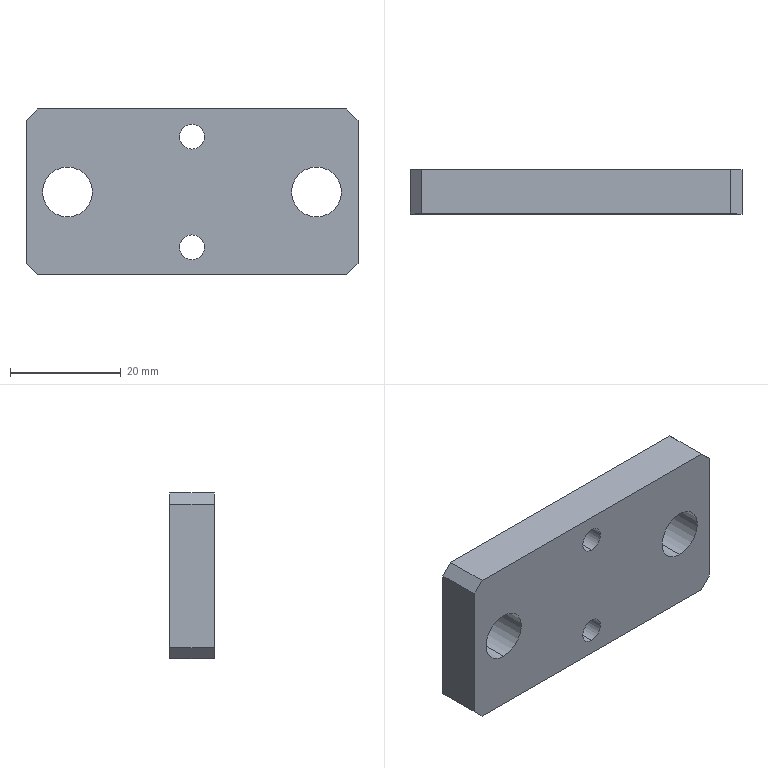Part | 1 solid | 24 faces | box 60 x 8 x 30 mm | volume 12748 mm3 | cylinder 12 | plane 12 | commonest cylinder face diameters 4.5 x4 8 x4 9 x4
STEP:
#1=CARTESIAN_POINT('',(22.5,4.,4.5));
#2=VERTEX_POINT('',#1);
#3=CARTESIAN_POINT('',(22.5,4.,-4.5));
#4=VERTEX_POINT('',#3);
#5=CARTESIAN_POINT('',(22.5,4.,0.));
#6=DIRECTION('',(0.,-1.,0.));
#7=DIRECTION('',(0.,0.,-1.));
#8=AXIS2_PLACEMENT_3D('',#5,#6,#7);
#9=CIRCLE('',#8,4.5);
#10=EDGE_CURVE('',#2,#4,#9,.T.);
#11=ORIENTED_EDGE('',*,*,#10,.F.);
#12=CARTESIAN_POINT('',(22.5,-4.,4.5));
#13=VERTEX_POINT('',#12);
#14=CARTESIAN_POINT('',(22.5,-4.,4.5));
#15=DIRECTION('',(0.,-1.,0.));
#16=VECTOR('',#15,1000.);
#17=LINE('',#14,#16);
#18=EDGE_CURVE('',#2,#13,#17,.T.);
#19=ORIENTED_EDGE('',*,*,#18,.T.);
#20=CARTESIAN_POINT('',(22.5,-4.,-4.5));
#21=VERTEX_POINT('',#20);
#22=CARTESIAN_POINT('',(22.5,-4.,0.));
#23=DIRECTION('',(0.,-1.,0.));
#24=DIRECTION('',(0.,0.,-1.));
#25=AXIS2_PLACEMENT_3D('',#22,#23,#24);
#26=CIRCLE('',#25,4.5);
#27=EDGE_CURVE('',#13,#21,#26,.T.);
#28=ORIENTED_EDGE('',*,*,#27,.T.);
#29=CARTESIAN_POINT('',(22.5,-4.,-4.5));
#30=DIRECTION('',(0.,-1.,0.));
#31=VECTOR('',#30,1000.);
#32=LINE('',#29,#31);
#33=EDGE_CURVE('',#4,#21,#32,.T.);
#34=ORIENTED_EDGE('',*,*,#33,.F.);
#35=EDGE_LOOP('',(#11,#19,#28,#34));
#36=FACE_OUTER_BOUND('',#35,.T.);
#37=CARTESIAN_POINT('',(22.5,-4.,0.));
#38=DIRECTION('',(0.,-1.,0.));
#39=DIRECTION('',(0.,0.,-1.));
#40=AXIS2_PLACEMENT_3D('',#37,#38,#39);
#41=CYLINDRICAL_SURFACE('',#40,4.5);
#42=ADVANCED_FACE('',(#36),#41,.F.);
#43=CARTESIAN_POINT('',(-22.5,4.,4.5));
#44=VERTEX_POINT('',#43);
#45=CARTESIAN_POINT('',(-22.5,4.,-4.5));
#46=VERTEX_POINT('',#45);
#47=CARTESIAN_POINT('',(-22.5,4.,0.));
#48=DIRECTION('',(0.,-1.,0.));
#49=DIRECTION('',(0.,0.,-1.));
#50=AXIS2_PLACEMENT_3D('',#47,#48,#49);
#51=CIRCLE('',#50,4.5);
#52=EDGE_CURVE('',#44,#46,#51,.T.);
#53=ORIENTED_EDGE('',*,*,#52,.F.);
#54=CARTESIAN_POINT('',(-22.5,-4.,4.5));
#55=VERTEX_POINT('',#54);
#56=CARTESIAN_POINT('',(-22.5,-4.,4.5));
#57=DIRECTION('',(0.,-1.,0.));
#58=VECTOR('',#57,1000.);
#59=LINE('',#56,#58);
#60=EDGE_CURVE('',#44,#55,#59,.T.);
#61=ORIENTED_EDGE('',*,*,#60,.T.);
#62=CARTESIAN_POINT('',(-22.5,-4.,-4.5));
#63=VERTEX_POINT('',#62);
#64=CARTESIAN_POINT('',(-22.5,-4.,0.));
#65=DIRECTION('',(0.,-1.,0.));
#66=DIRECTION('',(0.,0.,-1.));
#67=AXIS2_PLACEMENT_3D('',#64,#65,#66);
#68=CIRCLE('',#67,4.5);
#69=EDGE_CURVE('',#55,#63,#68,.T.);
#70=ORIENTED_EDGE('',*,*,#69,.T.);
#71=CARTESIAN_POINT('',(-22.5,-4.,-4.5));
#72=DIRECTION('',(0.,-1.,0.));
#73=VECTOR('',#72,1000.);
#74=LINE('',#71,#73);
#75=EDGE_CURVE('',#46,#63,#74,.T.);
#76=ORIENTED_EDGE('',*,*,#75,.F.);
#77=EDGE_LOOP('',(#53,#61,#70,#76));
#78=FACE_OUTER_BOUND('',#77,.T.);
#79=CARTESIAN_POINT('',(-22.5,-4.,0.));
#80=DIRECTION('',(0.,-1.,0.));
#81=DIRECTION('',(0.,0.,-1.));
#82=AXIS2_PLACEMENT_3D('',#79,#80,#81);
#83=CYLINDRICAL_SURFACE('',#82,4.5);
#84=ADVANCED_FACE('',(#78),#83,.F.);
#85=CARTESIAN_POINT('',(0.,-0.6,6.));
#86=VERTEX_POINT('',#85);
#87=CARTESIAN_POINT('',(0.,-0.6,14.));
#88=VERTEX_POINT('',#87);
#89=CARTESIAN_POINT('',(0.,-0.6,10.));
#90=DIRECTION('',(0.,1.,0.));
#91=DIRECTION('',(0.,0.,1.));
#92=AXIS2_PLACEMENT_3D('',#89,#90,#91);
#93=CIRCLE('',#92,4.);
#94=EDGE_CURVE('',#86,#88,#93,.T.);
#95=ORIENTED_EDGE('',*,*,#94,.F.);
#96=CARTESIAN_POINT('',(0.,4.,6.));
#97=VERTEX_POINT('',#96);
#98=CARTESIAN_POINT('',(0.,4.,6.));
#99=DIRECTION('',(0.,1.,0.));
#100=VECTOR('',#99,1000.);
#101=LINE('',#98,#100);
#102=EDGE_CURVE('',#86,#97,#101,.T.);
#103=ORIENTED_EDGE('',*,*,#102,.T.);
#104=CARTESIAN_POINT('',(0.,4.,14.));
#105=VERTEX_POINT('',#104);
#106=CARTESIAN_POINT('',(0.,4.,10.));
#107=DIRECTION('',(0.,1.,0.));
#108=DIRECTION('',(0.,0.,1.));
#109=AXIS2_PLACEMENT_3D('',#106,#107,#108);
#110=CIRCLE('',#109,4.);
#111=EDGE_CURVE('',#97,#105,#110,.T.);
#112=ORIENTED_EDGE('',*,*,#111,.T.);
#113=CARTESIAN_POINT('',(0.,4.,14.));
#114=DIRECTION('',(0.,1.,0.));
#115=VECTOR('',#114,1000.);
#116=LINE('',#113,#115);
#117=EDGE_CURVE('',#88,#105,#116,.T.);
#118=ORIENTED_EDGE('',*,*,#117,.F.);
#119=EDGE_LOOP('',(#95,#103,#112,#118));
#120=FACE_OUTER_BOUND('',#119,.T.);
#121=CARTESIAN_POINT('',(0.,4.,10.));
#122=DIRECTION('',(0.,1.,0.));
#123=DIRECTION('',(0.,0.,1.));
#124=AXIS2_PLACEMENT_3D('',#121,#122,#123);
#125=CYLINDRICAL_SURFACE('',#124,4.);
#126=ADVANCED_FACE('',(#120),#125,.F.);
#127=CARTESIAN_POINT('',(0.,-4.,7.75));
#128=VERTEX_POINT('',#127);
#129=CARTESIAN_POINT('',(0.,-4.,12.25));
#130=VERTEX_POINT('',#129);
#131=CARTESIAN_POINT('',(0.,-4.,10.));
#132=DIRECTION('',(0.,1.,0.));
#133=DIRECTION('',(0.,0.,1.));
#134=AXIS2_PLACEMENT_3D('',#131,#132,#133);
#135=CIRCLE('',#134,2.25);
#136=EDGE_CURVE('',#128,#130,#135,.T.);
#137=ORIENTED_EDGE('',*,*,#136,.F.);
#138=CARTESIAN_POINT('',(0.,-0.6,7.75));
#139=VERTEX_POINT('',#138);
#140=CARTESIAN_POINT('',(0.,4.,7.75));
#141=DIRECTION('',(0.,1.,0.));
#142=VECTOR('',#141,1000.);
#143=LINE('',#140,#142);
#144=EDGE_CURVE('',#128,#139,#143,.T.);
#145=ORIENTED_EDGE('',*,*,#144,.T.);
#146=CARTESIAN_POINT('',(0.,-0.6,12.25));
#147=VERTEX_POINT('',#146);
#148=CARTESIAN_POINT('',(0.,-0.6,10.));
#149=DIRECTION('',(0.,1.,0.));
#150=DIRECTION('',(0.,0.,1.));
#151=AXIS2_PLACEMENT_3D('',#148,#149,#150);
#152=CIRCLE('',#151,2.25);
#153=EDGE_CURVE('',#139,#147,#152,.T.);
#154=ORIENTED_EDGE('',*,*,#153,.T.);
#155=CARTESIAN_POINT('',(0.,4.,12.25));
#156=DIRECTION('',(0.,1.,0.));
#157=VECTOR('',#156,1000.);
#158=LINE('',#155,#157);
#159=EDGE_CURVE('',#130,#147,#158,.T.);
#160=ORIENTED_EDGE('',*,*,#159,.F.);
#161=EDGE_LOOP('',(#137,#145,#154,#160));
#162=FACE_OUTER_BOUND('',#161,.T.);
#163=CARTESIAN_POINT('',(0.,4.,10.));
#164=DIRECTION('',(0.,1.,0.));
#165=DIRECTION('',(0.,0.,1.));
#166=AXIS2_PLACEMENT_3D('',#163,#164,#165);
#167=CYLINDRICAL_SURFACE('',#166,2.25);
#168=ADVANCED_FACE('',(#162),#167,.F.);
#169=CARTESIAN_POINT('',(0.,-0.6,-14.));
#170=VERTEX_POINT('',#169);
#171=CARTESIAN_POINT('',(0.,-0.6,-6.));
#172=VERTEX_POINT('',#171);
#173=CARTESIAN_POINT('',(0.,-0.6,-10.));
#174=DIRECTION('',(0.,1.,0.));
#175=DIRECTION('',(0.,0.,1.));
#176=AXIS2_PLACEMENT_3D('',#173,#174,#175);
#177=CIRCLE('',#176,4.);
#178=EDGE_CURVE('',#170,#172,#177,.T.);
#179=ORIENTED_EDGE('',*,*,#178,.F.);
#180=CARTESIAN_POINT('',(0.,4.,-14.));
#181=VERTEX_POINT('',#180);
#182=CARTESIAN_POINT('',(0.,4.,-14.));
#183=DIRECTION('',(0.,1.,0.));
#184=VECTOR('',#183,1000.);
#185=LINE('',#182,#184);
#186=EDGE_CURVE('',#170,#181,#185,.T.);
#187=ORIENTED_EDGE('',*,*,#186,.T.);
#188=CARTESIAN_POINT('',(0.,4.,-6.));
#189=VERTEX_POINT('',#188);
#190=CARTESIAN_POINT('',(0.,4.,-10.));
#191=DIRECTION('',(0.,1.,0.));
#192=DIRECTION('',(0.,0.,1.));
#193=AXIS2_PLACEMENT_3D('',#190,#191,#192);
#194=CIRCLE('',#193,4.);
#195=EDGE_CURVE('',#181,#189,#194,.T.);
#196=ORIENTED_EDGE('',*,*,#195,.T.);
#197=CARTESIAN_POINT('',(0.,4.,-6.));
#198=DIRECTION('',(0.,1.,0.));
#199=VECTOR('',#198,1000.);
#200=LINE('',#197,#199);
#201=EDGE_CURVE('',#172,#189,#200,.T.);
#202=ORIENTED_EDGE('',*,*,#201,.F.);
#203=EDGE_LOOP('',(#179,#187,#196,#202));
#204=FACE_OUTER_BOUND('',#203,.T.);
#205=CARTESIAN_POINT('',(0.,4.,-10.));
#206=DIRECTION('',(0.,1.,0.));
#207=DIRECTION('',(0.,0.,1.));
#208=AXIS2_PLACEMENT_3D('',#205,#206,#207);
#209=CYLINDRICAL_SURFACE('',#208,4.);
#210=ADVANCED_FACE('',(#204),#209,.F.);
#211=CARTESIAN_POINT('',(0.,-4.,-12.25));
#212=VERTEX_POINT('',#211);
#213=CARTESIAN_POINT('',(0.,-4.,-7.75));
#214=VERTEX_POINT('',#213);
#215=CARTESIAN_POINT('',(0.,-4.,-10.));
#216=DIRECTION('',(0.,1.,0.));
#217=DIRECTION('',(0.,0.,1.));
#218=AXIS2_PLACEMENT_3D('',#215,#216,#217);
#219=CIRCLE('',#218,2.25);
#220=EDGE_CURVE('',#212,#214,#219,.T.);
#221=ORIENTED_EDGE('',*,*,#220,.F.);
#222=CARTESIAN_POINT('',(0.,-0.6,-12.25));
#223=VERTEX_POINT('',#222);
#224=CARTESIAN_POINT('',(0.,4.,-12.25));
#225=DIRECTION('',(0.,1.,0.));
#226=VECTOR('',#225,1000.);
#227=LINE('',#224,#226);
#228=EDGE_CURVE('',#212,#223,#227,.T.);
#229=ORIENTED_EDGE('',*,*,#228,.T.);
#230=CARTESIAN_POINT('',(0.,-0.6,-7.75));
#231=VERTEX_POINT('',#230);
#232=CARTESIAN_POINT('',(0.,-0.6,-10.));
#233=DIRECTION('',(0.,1.,0.));
#234=DIRECTION('',(0.,0.,1.));
#235=AXIS2_PLACEMENT_3D('',#232,#233,#234);
#236=CIRCLE('',#235,2.25);
#237=EDGE_CURVE('',#223,#231,#236,.T.);
#238=ORIENTED_EDGE('',*,*,#237,.T.);
#239=CARTESIAN_POINT('',(0.,4.,-7.75));
#240=DIRECTION('',(0.,1.,0.));
#241=VECTOR('',#240,1000.);
#242=LINE('',#239,#241);
#243=EDGE_CURVE('',#214,#231,#242,.T.);
#244=ORIENTED_EDGE('',*,*,#243,.F.);
#245=EDGE_LOOP('',(#221,#229,#238,#244));
#246=FACE_OUTER_BOUND('',#245,.T.);
#247=CARTESIAN_POINT('',(0.,4.,-10.));
#248=DIRECTION('',(0.,1.,0.));
#249=DIRECTION('',(0.,0.,1.));
#250=AXIS2_PLACEMENT_3D('',#247,#248,#249);
#251=CYLINDRICAL_SURFACE('',#250,2.25);
#252=ADVANCED_FACE('',(#246),#251,.F.);
#253=CARTESIAN_POINT('',(30.,4.,13.));
#254=VERTEX_POINT('',#253);
#255=CARTESIAN_POINT('',(30.,4.,-13.));
#256=VERTEX_POINT('',#255);
#257=CARTESIAN_POINT('',(30.,4.,15.));
#258=DIRECTION('',(0.,0.,-1.));
#259=VECTOR('',#258,1000.);
#260=LINE('',#257,#259);
#261=EDGE_CURVE('',#254,#256,#260,.T.);
#262=ORIENTED_EDGE('',*,*,#261,.F.);
#263=CARTESIAN_POINT('',(30.,-4.,13.));
#264=VERTEX_POINT('',#263);
#265=CARTESIAN_POINT('',(30.,4.,13.));
#266=DIRECTION('',(0.,-1.,0.));
#267=VECTOR('',#266,1000.);
#268=LINE('',#265,#267);
#269=EDGE_CURVE('',#254,#264,#268,.T.);
#270=ORIENTED_EDGE('',*,*,#269,.T.);
#271=CARTESIAN_POINT('',(30.,-4.,-13.));
#272=VERTEX_POINT('',#271);
#273=CARTESIAN_POINT('',(30.,-4.,15.));
#274=DIRECTION('',(0.,0.,-1.));
#275=VECTOR('',#274,1000.);
#276=LINE('',#273,#275);
#277=EDGE_CURVE('',#264,#272,#276,.T.);
#278=ORIENTED_EDGE('',*,*,#277,.T.);
#279=CARTESIAN_POINT('',(30.,4.,-13.));
#280=DIRECTION('',(0.,1.,0.));
#281=VECTOR('',#280,1000.);
#282=LINE('',#279,#281);
#283=EDGE_CURVE('',#272,#256,#282,.T.);
#284=ORIENTED_EDGE('',*,*,#283,.T.);
#285=EDGE_LOOP('',(#262,#270,#278,#284));
#286=FACE_OUTER_BOUND('',#285,.T.);
#287=CARTESIAN_POINT('',(30.,4.,15.));
#288=DIRECTION('',(-1.,0.,0.));
#289=DIRECTION('',(0.,0.,1.));
#290=AXIS2_PLACEMENT_3D('',#287,#288,#289);
#291=PLANE('',#290);
#292=ADVANCED_FACE('',(#286),#291,.F.);
#293=CARTESIAN_POINT('',(28.,-4.,-15.));
#294=VERTEX_POINT('',#293);
#295=CARTESIAN_POINT('',(-28.,-4.,-15.));
#296=VERTEX_POINT('',#295);
#297=CARTESIAN_POINT('',(-30.,-4.,-15.));
#298=DIRECTION('',(-1.,0.,0.));
#299=VECTOR('',#298,1000.);
#300=LINE('',#297,#299);
#301=EDGE_CURVE('',#294,#296,#300,.T.);
#302=ORIENTED_EDGE('',*,*,#301,.T.);
#303=CARTESIAN_POINT('',(-28.,4.,-15.));
#304=VERTEX_POINT('',#303);
#305=CARTESIAN_POINT('',(-28.,4.,-15.));
#306=DIRECTION('',(0.,1.,0.));
#307=VECTOR('',#306,1000.);
#308=LINE('',#305,#307);
#309=EDGE_CURVE('',#296,#304,#308,.T.);
#310=ORIENTED_EDGE('',*,*,#309,.T.);
#311=CARTESIAN_POINT('',(28.,4.,-15.));
#312=VERTEX_POINT('',#311);
#313=CARTESIAN_POINT('',(-30.,4.,-15.));
#314=DIRECTION('',(-1.,0.,0.));
#315=VECTOR('',#314,1000.);
#316=LINE('',#313,#315);
#317=EDGE_CURVE('',#312,#304,#316,.T.);
#318=ORIENTED_EDGE('',*,*,#317,.F.);
#319=CARTESIAN_POINT('',(28.,4.,-15.));
#320=DIRECTION('',(0.,-1.,0.));
#321=VECTOR('',#320,1000.);
#322=LINE('',#319,#321);
#323=EDGE_CURVE('',#312,#294,#322,.T.);
#324=ORIENTED_EDGE('',*,*,#323,.T.);
#325=EDGE_LOOP('',(#302,#310,#318,#324));
#326=FACE_OUTER_BOUND('',#325,.T.);
#327=CARTESIAN_POINT('',(-30.,4.,-15.));
#328=DIRECTION('',(0.,0.,1.));
#329=DIRECTION('',(1.,0.,0.));
#330=AXIS2_PLACEMENT_3D('',#327,#328,#329);
#331=PLANE('',#330);
#332=ADVANCED_FACE('',(#326),#331,.F.);
#333=CARTESIAN_POINT('',(-30.,-4.,-13.));
#334=VERTEX_POINT('',#333);
#335=CARTESIAN_POINT('',(-30.,-4.,13.));
#336=VERTEX_POINT('',#335);
#337=CARTESIAN_POINT('',(-30.,-4.,15.));
#338=DIRECTION('',(0.,0.,1.));
#339=VECTOR('',#338,1000.);
#340=LINE('',#337,#339);
#341=EDGE_CURVE('',#334,#336,#340,.T.);
#342=ORIENTED_EDGE('',*,*,#341,.T.);
#343=CARTESIAN_POINT('',(-30.,4.,13.));
#344=VERTEX_POINT('',#343);
#345=CARTESIAN_POINT('',(-30.,4.,13.));
#346=DIRECTION('',(0.,1.,0.));
#347=VECTOR('',#346,1000.);
#348=LINE('',#345,#347);
#349=EDGE_CURVE('',#336,#344,#348,.T.);
#350=ORIENTED_EDGE('',*,*,#349,.T.);
#351=CARTESIAN_POINT('',(-30.,4.,-13.));
#352=VERTEX_POINT('',#351);
#353=CARTESIAN_POINT('',(-30.,4.,15.));
#354=DIRECTION('',(0.,0.,1.));
#355=VECTOR('',#354,1000.);
#356=LINE('',#353,#355);
#357=EDGE_CURVE('',#352,#344,#356,.T.);
#358=ORIENTED_EDGE('',*,*,#357,.F.);
#359=CARTESIAN_POINT('',(-30.,4.,-13.));
#360=DIRECTION('',(0.,-1.,0.));
#361=VECTOR('',#360,1000.);
#362=LINE('',#359,#361);
#363=EDGE_CURVE('',#352,#334,#362,.T.);
#364=ORIENTED_EDGE('',*,*,#363,.T.);
#365=EDGE_LOOP('',(#342,#350,#358,#364));
#366=FACE_OUTER_BOUND('',#365,.T.);
#367=CARTESIAN_POINT('',(-30.,4.,15.));
#368=DIRECTION('',(1.,0.,0.));
#369=DIRECTION('',(0.,0.,-1.));
#370=AXIS2_PLACEMENT_3D('',#367,#368,#369);
#371=PLANE('',#370);
#372=ADVANCED_FACE('',(#366),#371,.F.);
#373=CARTESIAN_POINT('',(-28.,4.,15.));
#374=VERTEX_POINT('',#373);
#375=CARTESIAN_POINT('',(28.,4.,15.));
#376=VERTEX_POINT('',#375);
#377=CARTESIAN_POINT('',(-30.,4.,15.));
#378=DIRECTION('',(1.,0.,0.));
#379=VECTOR('',#378,1000.);
#380=LINE('',#377,#379);
#381=EDGE_CURVE('',#374,#376,#380,.T.);
#382=ORIENTED_EDGE('',*,*,#381,.F.);
#383=CARTESIAN_POINT('',(-28.,-4.,15.));
#384=VERTEX_POINT('',#383);
#385=CARTESIAN_POINT('',(-28.,4.,15.));
#386=DIRECTION('',(0.,-1.,0.));
#387=VECTOR('',#386,1000.);
#388=LINE('',#385,#387);
#389=EDGE_CURVE('',#374,#384,#388,.T.);
#390=ORIENTED_EDGE('',*,*,#389,.T.);
#391=CARTESIAN_POINT('',(28.,-4.,15.));
#392=VERTEX_POINT('',#391);
#393=CARTESIAN_POINT('',(-30.,-4.,15.));
#394=DIRECTION('',(1.,0.,0.));
#395=VECTOR('',#394,1000.);
#396=LINE('',#393,#395);
#397=EDGE_CURVE('',#384,#392,#396,.T.);
#398=ORIENTED_EDGE('',*,*,#397,.T.);
#399=CARTESIAN_POINT('',(28.,4.,15.));
#400=DIRECTION('',(0.,1.,0.));
#401=VECTOR('',#400,1000.);
#402=LINE('',#399,#401);
#403=EDGE_CURVE('',#392,#376,#402,.T.);
#404=ORIENTED_EDGE('',*,*,#403,.T.);
#405=EDGE_LOOP('',(#382,#390,#398,#404));
#406=FACE_OUTER_BOUND('',#405,.T.);
#407=CARTESIAN_POINT('',(-30.,4.,15.));
#408=DIRECTION('',(0.,0.,-1.));
#409=DIRECTION('',(-1.,0.,0.));
#410=AXIS2_PLACEMENT_3D('',#407,#408,#409);
#411=PLANE('',#410);
#412=ADVANCED_FACE('',(#406),#411,.F.);
#413=CARTESIAN_POINT('',(22.5,4.,0.));
#414=DIRECTION('',(0.,-1.,0.));
#415=DIRECTION('',(0.,0.,-1.));
#416=AXIS2_PLACEMENT_3D('',#413,#414,#415);
#417=CIRCLE('',#416,4.5);
#418=EDGE_CURVE('',#4,#2,#417,.T.);
#419=ORIENTED_EDGE('',*,*,#418,.T.);
#420=ORIENTED_EDGE('',*,*,#10,.T.);
#421=EDGE_LOOP('',(#419,#420));
#422=FACE_BOUND('',#421,.T.);
#423=CARTESIAN_POINT('',(-22.5,4.,0.));
#424=DIRECTION('',(0.,-1.,0.));
#425=DIRECTION('',(0.,0.,-1.));
#426=AXIS2_PLACEMENT_3D('',#423,#424,#425);
#427=CIRCLE('',#426,4.5);
#428=EDGE_CURVE('',#46,#44,#427,.T.);
#429=ORIENTED_EDGE('',*,*,#428,.T.);
#430=ORIENTED_EDGE('',*,*,#52,.T.);
#431=EDGE_LOOP('',(#429,#430));
#432=FACE_BOUND('',#431,.T.);
#433=CARTESIAN_POINT('',(0.,4.,10.));
#434=DIRECTION('',(0.,1.,0.));
#435=DIRECTION('',(0.,0.,1.));
#436=AXIS2_PLACEMENT_3D('',#433,#434,#435);
#437=CIRCLE('',#436,4.);
#438=EDGE_CURVE('',#105,#97,#437,.T.);
#439=ORIENTED_EDGE('',*,*,#438,.F.);
#440=ORIENTED_EDGE('',*,*,#111,.F.);
#441=EDGE_LOOP('',(#439,#440));
#442=FACE_BOUND('',#441,.T.);
#443=CARTESIAN_POINT('',(0.,4.,-10.));
#444=DIRECTION('',(0.,1.,0.));
#445=DIRECTION('',(0.,0.,1.));
#446=AXIS2_PLACEMENT_3D('',#443,#444,#445);
#447=CIRCLE('',#446,4.);
#448=EDGE_CURVE('',#189,#181,#447,.T.);
#449=ORIENTED_EDGE('',*,*,#448,.F.);
#450=ORIENTED_EDGE('',*,*,#195,.F.);
#451=EDGE_LOOP('',(#449,#450));
#452=FACE_BOUND('',#451,.T.);
#453=ORIENTED_EDGE('',*,*,#357,.T.);
#454=CARTESIAN_POINT('',(-28.,4.,15.));
#455=DIRECTION('',(0.7071,0.,0.7071));
#456=VECTOR('',#455,1000.);
#457=LINE('',#454,#456);
#458=EDGE_CURVE('',#344,#374,#457,.T.);
#459=ORIENTED_EDGE('',*,*,#458,.T.);
#460=ORIENTED_EDGE('',*,*,#381,.T.);
#461=CARTESIAN_POINT('',(30.,4.,13.));
#462=DIRECTION('',(0.7071,0.,-0.7071));
#463=VECTOR('',#462,1000.);
#464=LINE('',#461,#463);
#465=EDGE_CURVE('',#376,#254,#464,.T.);
#466=ORIENTED_EDGE('',*,*,#465,.T.);
#467=ORIENTED_EDGE('',*,*,#261,.T.);
#468=CARTESIAN_POINT('',(28.,4.,-15.));
#469=DIRECTION('',(-0.7071,0.,-0.7071));
#470=VECTOR('',#469,1000.);
#471=LINE('',#468,#470);
#472=EDGE_CURVE('',#256,#312,#471,.T.);
#473=ORIENTED_EDGE('',*,*,#472,.T.);
#474=ORIENTED_EDGE('',*,*,#317,.T.);
#475=CARTESIAN_POINT('',(-30.,4.,-13.));
#476=DIRECTION('',(-0.7071,0.,0.7071));
#477=VECTOR('',#476,1000.);
#478=LINE('',#475,#477);
#479=EDGE_CURVE('',#304,#352,#478,.T.);
#480=ORIENTED_EDGE('',*,*,#479,.T.);
#481=EDGE_LOOP('',(#453,#459,#460,#466,#467,#473,#474,#480));
#482=FACE_OUTER_BOUND('',#481,.T.);
#483=CARTESIAN_POINT('',(0.,4.,0.));
#484=DIRECTION('',(0.,-1.,0.));
#485=DIRECTION('',(0.,0.,-1.));
#486=AXIS2_PLACEMENT_3D('',#483,#484,#485);
#487=PLANE('',#486);
#488=ADVANCED_FACE('',(#422,#432,#442,#452,#482),#487,.F.);
#489=CARTESIAN_POINT('',(22.5,-4.,0.));
#490=DIRECTION('',(0.,-1.,0.));
#491=DIRECTION('',(0.,0.,-1.));
#492=AXIS2_PLACEMENT_3D('',#489,#490,#491);
#493=CIRCLE('',#492,4.5);
#494=EDGE_CURVE('',#21,#13,#493,.T.);
#495=ORIENTED_EDGE('',*,*,#494,.F.);
#496=ORIENTED_EDGE('',*,*,#27,.F.);
#497=EDGE_LOOP('',(#495,#496));
#498=FACE_BOUND('',#497,.T.);
#499=CARTESIAN_POINT('',(-22.5,-4.,0.));
#500=DIRECTION('',(0.,-1.,0.));
#501=DIRECTION('',(0.,0.,-1.));
#502=AXIS2_PLACEMENT_3D('',#499,#500,#501);
#503=CIRCLE('',#502,4.5);
#504=EDGE_CURVE('',#63,#55,#503,.T.);
#505=ORIENTED_EDGE('',*,*,#504,.F.);
#506=ORIENTED_EDGE('',*,*,#69,.F.);
#507=EDGE_LOOP('',(#505,#506));
#508=FACE_BOUND('',#507,.T.);
#509=CARTESIAN_POINT('',(0.,-4.,10.));
#510=DIRECTION('',(0.,1.,0.));
#511=DIRECTION('',(0.,0.,1.));
#512=AXIS2_PLACEMENT_3D('',#509,#510,#511);
#513=CIRCLE('',#512,2.25);
#514=EDGE_CURVE('',#130,#128,#513,.T.);
#515=ORIENTED_EDGE('',*,*,#514,.T.);
#516=ORIENTED_EDGE('',*,*,#136,.T.);
#517=EDGE_LOOP('',(#515,#516));
#518=FACE_BOUND('',#517,.T.);
#519=CARTESIAN_POINT('',(0.,-4.,-10.));
#520=DIRECTION('',(0.,1.,0.));
#521=DIRECTION('',(0.,0.,1.));
#522=AXIS2_PLACEMENT_3D('',#519,#520,#521);
#523=CIRCLE('',#522,2.25);
#524=EDGE_CURVE('',#214,#212,#523,.T.);
#525=ORIENTED_EDGE('',*,*,#524,.T.);
#526=ORIENTED_EDGE('',*,*,#220,.T.);
#527=EDGE_LOOP('',(#525,#526));
#528=FACE_BOUND('',#527,.T.);
#529=ORIENTED_EDGE('',*,*,#397,.F.);
#530=CARTESIAN_POINT('',(-21.5,-4.,21.5));
#531=DIRECTION('',(-0.7071,0.,-0.7071));
#532=VECTOR('',#531,1000.);
#533=LINE('',#530,#532);
#534=EDGE_CURVE('',#384,#336,#533,.T.);
#535=ORIENTED_EDGE('',*,*,#534,.T.);
#536=ORIENTED_EDGE('',*,*,#341,.F.);
#537=CARTESIAN_POINT('',(-21.5,-4.,-21.5));
#538=DIRECTION('',(0.7071,0.,-0.7071));
#539=VECTOR('',#538,1000.);
#540=LINE('',#537,#539);
#541=EDGE_CURVE('',#334,#296,#540,.T.);
#542=ORIENTED_EDGE('',*,*,#541,.T.);
#543=ORIENTED_EDGE('',*,*,#301,.F.);
#544=CARTESIAN_POINT('',(21.5,-4.,-21.5));
#545=DIRECTION('',(0.7071,0.,0.7071));
#546=VECTOR('',#545,1000.);
#547=LINE('',#544,#546);
#548=EDGE_CURVE('',#294,#272,#547,.T.);
#549=ORIENTED_EDGE('',*,*,#548,.T.);
#550=ORIENTED_EDGE('',*,*,#277,.F.);
#551=CARTESIAN_POINT('',(21.5,-4.,21.5));
#552=DIRECTION('',(-0.7071,0.,0.7071));
#553=VECTOR('',#552,1000.);
#554=LINE('',#551,#553);
#555=EDGE_CURVE('',#264,#392,#554,.T.);
#556=ORIENTED_EDGE('',*,*,#555,.T.);
#557=EDGE_LOOP('',(#529,#535,#536,#542,#543,#549,#550,#556));
#558=FACE_OUTER_BOUND('',#557,.T.);
#559=CARTESIAN_POINT('',(0.,-4.,0.));
#560=DIRECTION('',(0.,-1.,0.));
#561=DIRECTION('',(0.,0.,-1.));
#562=AXIS2_PLACEMENT_3D('',#559,#560,#561);
#563=PLANE('',#562);
#564=ADVANCED_FACE('',(#498,#508,#518,#528,#558),#563,.T.);
#565=ORIENTED_EDGE('',*,*,#458,.F.);
#566=ORIENTED_EDGE('',*,*,#349,.F.);
#567=ORIENTED_EDGE('',*,*,#534,.F.);
#568=ORIENTED_EDGE('',*,*,#389,.F.);
#569=EDGE_LOOP('',(#565,#566,#567,#568));
#570=FACE_OUTER_BOUND('',#569,.T.);
#571=CARTESIAN_POINT('',(-28.,4.,15.));
#572=DIRECTION('',(0.7071,0.,-0.7071));
#573=DIRECTION('',(0.,-1.,0.));
#574=AXIS2_PLACEMENT_3D('',#571,#572,#573);
#575=PLANE('',#574);
#576=ADVANCED_FACE('',(#570),#575,.F.);
#577=ORIENTED_EDGE('',*,*,#479,.F.);
#578=ORIENTED_EDGE('',*,*,#309,.F.);
#579=ORIENTED_EDGE('',*,*,#541,.F.);
#580=ORIENTED_EDGE('',*,*,#363,.F.);
#581=EDGE_LOOP('',(#577,#578,#579,#580));
#582=FACE_OUTER_BOUND('',#581,.T.);
#583=CARTESIAN_POINT('',(-30.,4.,-13.));
#584=DIRECTION('',(0.7071,0.,0.7071));
#585=DIRECTION('',(0.,-1.,0.));
#586=AXIS2_PLACEMENT_3D('',#583,#584,#585);
#587=PLANE('',#586);
#588=ADVANCED_FACE('',(#582),#587,.F.);
#589=ORIENTED_EDGE('',*,*,#465,.F.);
#590=ORIENTED_EDGE('',*,*,#403,.F.);
#591=ORIENTED_EDGE('',*,*,#555,.F.);
#592=ORIENTED_EDGE('',*,*,#269,.F.);
#593=EDGE_LOOP('',(#589,#590,#591,#592));
#594=FACE_OUTER_BOUND('',#593,.T.);
#595=CARTESIAN_POINT('',(30.,4.,13.));
#596=DIRECTION('',(-0.7071,0.,-0.7071));
#597=DIRECTION('',(0.,-1.,0.));
#598=AXIS2_PLACEMENT_3D('',#595,#596,#597);
#599=PLANE('',#598);
#600=ADVANCED_FACE('',(#594),#599,.F.);
#601=ORIENTED_EDGE('',*,*,#472,.F.);
#602=ORIENTED_EDGE('',*,*,#283,.F.);
#603=ORIENTED_EDGE('',*,*,#548,.F.);
#604=ORIENTED_EDGE('',*,*,#323,.F.);
#605=EDGE_LOOP('',(#601,#602,#603,#604));
#606=FACE_OUTER_BOUND('',#605,.T.);
#607=CARTESIAN_POINT('',(28.,4.,-15.));
#608=DIRECTION('',(-0.7071,0.,0.7071));
#609=DIRECTION('',(0.,-1.,0.));
#610=AXIS2_PLACEMENT_3D('',#607,#608,#609);
#611=PLANE('',#610);
#612=ADVANCED_FACE('',(#606),#611,.F.);
#613=ORIENTED_EDGE('',*,*,#228,.F.);
#614=ORIENTED_EDGE('',*,*,#524,.F.);
#615=ORIENTED_EDGE('',*,*,#243,.T.);
#616=CARTESIAN_POINT('',(0.,-0.6,-10.));
#617=DIRECTION('',(0.,1.,0.));
#618=DIRECTION('',(0.,0.,1.));
#619=AXIS2_PLACEMENT_3D('',#616,#617,#618);
#620=CIRCLE('',#619,2.25);
#621=EDGE_CURVE('',#231,#223,#620,.T.);
#622=ORIENTED_EDGE('',*,*,#621,.T.);
#623=EDGE_LOOP('',(#613,#614,#615,#622));
#624=FACE_OUTER_BOUND('',#623,.T.);
#625=CARTESIAN_POINT('',(0.,4.,-10.));
#626=DIRECTION('',(0.,1.,0.));
#627=DIRECTION('',(0.,0.,1.));
#628=AXIS2_PLACEMENT_3D('',#625,#626,#627);
#629=CYLINDRICAL_SURFACE('',#628,2.25);
#630=ADVANCED_FACE('',(#624),#629,.F.);
#631=ORIENTED_EDGE('',*,*,#621,.F.);
#632=ORIENTED_EDGE('',*,*,#237,.F.);
#633=EDGE_LOOP('',(#631,#632));
#634=FACE_BOUND('',#633,.T.);
#635=CARTESIAN_POINT('',(0.,-0.6,-10.));
#636=DIRECTION('',(0.,1.,0.));
#637=DIRECTION('',(0.,0.,1.));
#638=AXIS2_PLACEMENT_3D('',#635,#636,#637);
#639=CIRCLE('',#638,4.);
#640=EDGE_CURVE('',#172,#170,#639,.T.);
#641=ORIENTED_EDGE('',*,*,#640,.T.);
#642=ORIENTED_EDGE('',*,*,#178,.T.);
#643=EDGE_LOOP('',(#641,#642));
#644=FACE_OUTER_BOUND('',#643,.T.);
#645=CARTESIAN_POINT('',(2.25,-0.6,-10.));
#646=DIRECTION('',(0.,-1.,0.));
#647=DIRECTION('',(0.,0.,-1.));
#648=AXIS2_PLACEMENT_3D('',#645,#646,#647);
#649=PLANE('',#648);
#650=ADVANCED_FACE('',(#634,#644),#649,.F.);
#651=ORIENTED_EDGE('',*,*,#186,.F.);
#652=ORIENTED_EDGE('',*,*,#640,.F.);
#653=ORIENTED_EDGE('',*,*,#201,.T.);
#654=ORIENTED_EDGE('',*,*,#448,.T.);
#655=EDGE_LOOP('',(#651,#652,#653,#654));
#656=FACE_OUTER_BOUND('',#655,.T.);
#657=CARTESIAN_POINT('',(0.,4.,-10.));
#658=DIRECTION('',(0.,1.,0.));
#659=DIRECTION('',(0.,0.,1.));
#660=AXIS2_PLACEMENT_3D('',#657,#658,#659);
#661=CYLINDRICAL_SURFACE('',#660,4.);
#662=ADVANCED_FACE('',(#656),#661,.F.);
#663=ORIENTED_EDGE('',*,*,#144,.F.);
#664=ORIENTED_EDGE('',*,*,#514,.F.);
#665=ORIENTED_EDGE('',*,*,#159,.T.);
#666=CARTESIAN_POINT('',(0.,-0.6,10.));
#667=DIRECTION('',(0.,1.,0.));
#668=DIRECTION('',(0.,0.,1.));
#669=AXIS2_PLACEMENT_3D('',#666,#667,#668);
#670=CIRCLE('',#669,2.25);
#671=EDGE_CURVE('',#147,#139,#670,.T.);
#672=ORIENTED_EDGE('',*,*,#671,.T.);
#673=EDGE_LOOP('',(#663,#664,#665,#672));
#674=FACE_OUTER_BOUND('',#673,.T.);
#675=CARTESIAN_POINT('',(0.,4.,10.));
#676=DIRECTION('',(0.,1.,0.));
#677=DIRECTION('',(0.,0.,1.));
#678=AXIS2_PLACEMENT_3D('',#675,#676,#677);
#679=CYLINDRICAL_SURFACE('',#678,2.25);
#680=ADVANCED_FACE('',(#674),#679,.F.);
#681=ORIENTED_EDGE('',*,*,#671,.F.);
#682=ORIENTED_EDGE('',*,*,#153,.F.);
#683=EDGE_LOOP('',(#681,#682));
#684=FACE_BOUND('',#683,.T.);
#685=CARTESIAN_POINT('',(0.,-0.6,10.));
#686=DIRECTION('',(0.,1.,0.));
#687=DIRECTION('',(0.,0.,1.));
#688=AXIS2_PLACEMENT_3D('',#685,#686,#687);
#689=CIRCLE('',#688,4.);
#690=EDGE_CURVE('',#88,#86,#689,.T.);
#691=ORIENTED_EDGE('',*,*,#690,.T.);
#692=ORIENTED_EDGE('',*,*,#94,.T.);
#693=EDGE_LOOP('',(#691,#692));
#694=FACE_OUTER_BOUND('',#693,.T.);
#695=CARTESIAN_POINT('',(2.25,-0.6,10.));
#696=DIRECTION('',(0.,-1.,0.));
#697=DIRECTION('',(0.,0.,-1.));
#698=AXIS2_PLACEMENT_3D('',#695,#696,#697);
#699=PLANE('',#698);
#700=ADVANCED_FACE('',(#684,#694),#699,.F.);
#701=ORIENTED_EDGE('',*,*,#102,.F.);
#702=ORIENTED_EDGE('',*,*,#690,.F.);
#703=ORIENTED_EDGE('',*,*,#117,.T.);
#704=ORIENTED_EDGE('',*,*,#438,.T.);
#705=EDGE_LOOP('',(#701,#702,#703,#704));
#706=FACE_OUTER_BOUND('',#705,.T.);
#707=CARTESIAN_POINT('',(0.,4.,10.));
#708=DIRECTION('',(0.,1.,0.));
#709=DIRECTION('',(0.,0.,1.));
#710=AXIS2_PLACEMENT_3D('',#707,#708,#709);
#711=CYLINDRICAL_SURFACE('',#710,4.);
#712=ADVANCED_FACE('',(#706),#711,.F.);
#713=ORIENTED_EDGE('',*,*,#60,.F.);
#714=ORIENTED_EDGE('',*,*,#428,.F.);
#715=ORIENTED_EDGE('',*,*,#75,.T.);
#716=ORIENTED_EDGE('',*,*,#504,.T.);
#717=EDGE_LOOP('',(#713,#714,#715,#716));
#718=FACE_OUTER_BOUND('',#717,.T.);
#719=CARTESIAN_POINT('',(-22.5,-4.,0.));
#720=DIRECTION('',(0.,-1.,0.));
#721=DIRECTION('',(0.,0.,-1.));
#722=AXIS2_PLACEMENT_3D('',#719,#720,#721);
#723=CYLINDRICAL_SURFACE('',#722,4.5);
#724=ADVANCED_FACE('',(#718),#723,.F.);
#725=ORIENTED_EDGE('',*,*,#18,.F.);
#726=ORIENTED_EDGE('',*,*,#418,.F.);
#727=ORIENTED_EDGE('',*,*,#33,.T.);
#728=ORIENTED_EDGE('',*,*,#494,.T.);
#729=EDGE_LOOP('',(#725,#726,#727,#728));
#730=FACE_OUTER_BOUND('',#729,.T.);
#731=CARTESIAN_POINT('',(22.5,-4.,0.));
#732=DIRECTION('',(0.,-1.,0.));
#733=DIRECTION('',(0.,0.,-1.));
#734=AXIS2_PLACEMENT_3D('',#731,#732,#733);
#735=CYLINDRICAL_SURFACE('',#734,4.5);
#736=ADVANCED_FACE('',(#730),#735,.F.);
#737=CLOSED_SHELL('',(#42,#84,#126,#168,#210,#252,#292,#332,#372,#412,#488,#564,#576,#588,#600,#612,#630,#650,#662,#680,#700,#712,#724,#736));
#738=MANIFOLD_SOLID_BREP('',#737);
#739=CARTESIAN_POINT('',(0.,0.,0.));
#740=DIRECTION('',(0.,0.,1.));
#741=DIRECTION('',(1.,0.,0.));
#742=AXIS2_PLACEMENT_3D('',#739,#740,#741);
#743=(LENGTH_UNIT()NAMED_UNIT(*)SI_UNIT(.MILLI.,.METRE.));
#744=UNCERTAINTY_MEASURE_WITH_UNIT(LENGTH_MEASURE(0.00001),#743,'','');
#745=(NAMED_UNIT(*)PLANE_ANGLE_UNIT()SI_UNIT($,.RADIAN.));
#746=(NAMED_UNIT(*)SI_UNIT($,.STERADIAN.)SOLID_ANGLE_UNIT());
#747=(GEOMETRIC_REPRESENTATION_CONTEXT(3)GLOBAL_UNCERTAINTY_ASSIGNED_CONTEXT((#744))GLOBAL_UNIT_ASSIGNED_CONTEXT((#743,#745,#746))REPRESENTATION_CONTEXT('',''));
#748=ADVANCED_BREP_SHAPE_REPRESENTATION('',(#738,#742),#747);